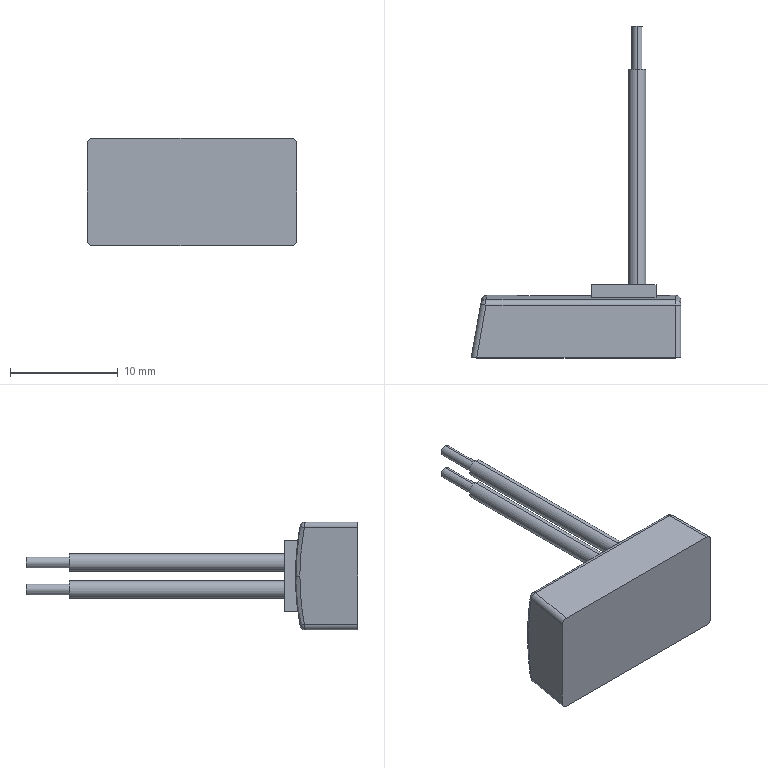Part | STEP file | 11-sy5120-5gz-01_v100 cover-V2.0-V2.011_G | 1 solid | 36 faces | box 19.45 x 30.8 x 10 mm | volume 1193 mm3 | cylinder 15 | plane 14 | sphere 4 | spline 2 | torus 1 | commonest cylinder face diameters 1 x10 1.6 x4 50 x1
STEP:
#1=CARTESIAN_POINT('',(-4.05,30.8,-0.75));
#2=VERTEX_POINT('',#1);
#3=CARTESIAN_POINT('',(-4.05,30.8,-1.75));
#4=VERTEX_POINT('',#3);
#5=CARTESIAN_POINT('',(-4.05,30.8,-1.25));
#6=DIRECTION('',(0.,1.,0.));
#7=DIRECTION('',(0.,0.,1.));
#8=AXIS2_PLACEMENT_3D('',#5,#6,#7);
#9=CIRCLE('',#8,0.5);
#10=EDGE_CURVE('',#2,#4,#9,.T.);
#11=ORIENTED_EDGE('',*,*,#10,.F.);
#12=CARTESIAN_POINT('',(-4.05,26.8,-0.75));
#13=VERTEX_POINT('',#12);
#14=CARTESIAN_POINT('',(-4.05,30.8,-0.75));
#15=DIRECTION('',(0.,-1.,0.));
#16=VECTOR('',#15,1000.);
#17=LINE('',#14,#16);
#18=EDGE_CURVE('',#2,#13,#17,.T.);
#19=ORIENTED_EDGE('',*,*,#18,.T.);
#20=CARTESIAN_POINT('',(-4.05,26.8,-1.75));
#21=VERTEX_POINT('',#20);
#22=CARTESIAN_POINT('',(-4.05,26.8,-1.25));
#23=DIRECTION('',(0.,1.,0.));
#24=DIRECTION('',(0.,0.,1.));
#25=AXIS2_PLACEMENT_3D('',#22,#23,#24);
#26=CIRCLE('',#25,0.5);
#27=EDGE_CURVE('',#13,#21,#26,.T.);
#28=ORIENTED_EDGE('',*,*,#27,.T.);
#29=CARTESIAN_POINT('',(-4.05,30.8,-1.75));
#30=DIRECTION('',(0.,-1.,0.));
#31=VECTOR('',#30,1000.);
#32=LINE('',#29,#31);
#33=EDGE_CURVE('',#4,#21,#32,.T.);
#34=ORIENTED_EDGE('',*,*,#33,.F.);
#35=EDGE_LOOP('',(#11,#19,#28,#34));
#36=FACE_OUTER_BOUND('',#35,.T.);
#37=CARTESIAN_POINT('',(-4.05,30.8,-1.25));
#38=DIRECTION('',(0.,-1.,0.));
#39=DIRECTION('',(0.,0.,-1.));
#40=AXIS2_PLACEMENT_3D('',#37,#38,#39);
#41=CYLINDRICAL_SURFACE('',#40,0.5);
#42=ADVANCED_FACE('',(#36),#41,.T.);
#43=CARTESIAN_POINT('',(-4.05,30.8,1.75));
#44=VERTEX_POINT('',#43);
#45=CARTESIAN_POINT('',(-4.05,30.8,0.75));
#46=VERTEX_POINT('',#45);
#47=CARTESIAN_POINT('',(-4.05,30.8,1.25));
#48=DIRECTION('',(0.,1.,0.));
#49=DIRECTION('',(0.,0.,1.));
#50=AXIS2_PLACEMENT_3D('',#47,#48,#49);
#51=CIRCLE('',#50,0.5);
#52=EDGE_CURVE('',#44,#46,#51,.T.);
#53=ORIENTED_EDGE('',*,*,#52,.F.);
#54=CARTESIAN_POINT('',(-4.05,26.8,1.75));
#55=VERTEX_POINT('',#54);
#56=CARTESIAN_POINT('',(-4.05,30.8,1.75));
#57=DIRECTION('',(0.,-1.,0.));
#58=VECTOR('',#57,1000.);
#59=LINE('',#56,#58);
#60=EDGE_CURVE('',#44,#55,#59,.T.);
#61=ORIENTED_EDGE('',*,*,#60,.T.);
#62=CARTESIAN_POINT('',(-4.05,26.8,0.75));
#63=VERTEX_POINT('',#62);
#64=CARTESIAN_POINT('',(-4.05,26.8,1.25));
#65=DIRECTION('',(0.,1.,0.));
#66=DIRECTION('',(0.,0.,1.));
#67=AXIS2_PLACEMENT_3D('',#64,#65,#66);
#68=CIRCLE('',#67,0.5);
#69=EDGE_CURVE('',#55,#63,#68,.T.);
#70=ORIENTED_EDGE('',*,*,#69,.T.);
#71=CARTESIAN_POINT('',(-4.05,30.8,0.75));
#72=DIRECTION('',(0.,-1.,0.));
#73=VECTOR('',#72,1000.);
#74=LINE('',#71,#73);
#75=EDGE_CURVE('',#46,#63,#74,.T.);
#76=ORIENTED_EDGE('',*,*,#75,.F.);
#77=EDGE_LOOP('',(#53,#61,#70,#76));
#78=FACE_OUTER_BOUND('',#77,.T.);
#79=CARTESIAN_POINT('',(-4.05,30.8,1.25));
#80=DIRECTION('',(0.,-1.,0.));
#81=DIRECTION('',(0.,0.,-1.));
#82=AXIS2_PLACEMENT_3D('',#79,#80,#81);
#83=CYLINDRICAL_SURFACE('',#82,0.5);
#84=ADVANCED_FACE('',(#78),#83,.T.);
#85=CARTESIAN_POINT('',(-4.05,26.8,-0.45));
#86=VERTEX_POINT('',#85);
#87=CARTESIAN_POINT('',(-4.05,26.8,-2.05));
#88=VERTEX_POINT('',#87);
#89=CARTESIAN_POINT('',(-4.05,26.8,-1.25));
#90=DIRECTION('',(0.,1.,0.));
#91=DIRECTION('',(0.,0.,1.));
#92=AXIS2_PLACEMENT_3D('',#89,#90,#91);
#93=CIRCLE('',#92,0.8);
#94=EDGE_CURVE('',#86,#88,#93,.T.);
#95=ORIENTED_EDGE('',*,*,#94,.F.);
#96=CARTESIAN_POINT('',(-4.05,6.8,-0.45));
#97=VERTEX_POINT('',#96);
#98=CARTESIAN_POINT('',(-4.05,26.8,-0.45));
#99=DIRECTION('',(0.,-1.,0.));
#100=VECTOR('',#99,1000.);
#101=LINE('',#98,#100);
#102=EDGE_CURVE('',#86,#97,#101,.T.);
#103=ORIENTED_EDGE('',*,*,#102,.T.);
#104=CARTESIAN_POINT('',(-4.05,6.8,-2.05));
#105=VERTEX_POINT('',#104);
#106=CARTESIAN_POINT('',(-4.05,6.8,-1.25));
#107=DIRECTION('',(0.,1.,0.));
#108=DIRECTION('',(0.,0.,-1.));
#109=AXIS2_PLACEMENT_3D('',#106,#107,#108);
#110=CIRCLE('',#109,0.8);
#111=EDGE_CURVE('',#97,#105,#110,.T.);
#112=ORIENTED_EDGE('',*,*,#111,.T.);
#113=CARTESIAN_POINT('',(-4.05,26.8,-2.05));
#114=DIRECTION('',(0.,-1.,0.));
#115=VECTOR('',#114,1000.);
#116=LINE('',#113,#115);
#117=EDGE_CURVE('',#88,#105,#116,.T.);
#118=ORIENTED_EDGE('',*,*,#117,.F.);
#119=EDGE_LOOP('',(#95,#103,#112,#118));
#120=FACE_OUTER_BOUND('',#119,.T.);
#121=CARTESIAN_POINT('',(-4.05,26.8,-1.25));
#122=DIRECTION('',(0.,-1.,0.));
#123=DIRECTION('',(0.,0.,-1.));
#124=AXIS2_PLACEMENT_3D('',#121,#122,#123);
#125=CYLINDRICAL_SURFACE('',#124,0.8);
#126=ADVANCED_FACE('',(#120),#125,.T.);
#127=CARTESIAN_POINT('',(-4.05,26.8,2.05));
#128=VERTEX_POINT('',#127);
#129=CARTESIAN_POINT('',(-4.05,26.8,0.45));
#130=VERTEX_POINT('',#129);
#131=CARTESIAN_POINT('',(-4.05,26.8,1.25));
#132=DIRECTION('',(0.,1.,0.));
#133=DIRECTION('',(0.,0.,1.));
#134=AXIS2_PLACEMENT_3D('',#131,#132,#133);
#135=CIRCLE('',#134,0.8);
#136=EDGE_CURVE('',#128,#130,#135,.T.);
#137=ORIENTED_EDGE('',*,*,#136,.F.);
#138=CARTESIAN_POINT('',(-4.05,6.8,2.05));
#139=VERTEX_POINT('',#138);
#140=CARTESIAN_POINT('',(-4.05,26.8,2.05));
#141=DIRECTION('',(0.,-1.,0.));
#142=VECTOR('',#141,1000.);
#143=LINE('',#140,#142);
#144=EDGE_CURVE('',#128,#139,#143,.T.);
#145=ORIENTED_EDGE('',*,*,#144,.T.);
#146=CARTESIAN_POINT('',(-4.05,6.8,0.45));
#147=VERTEX_POINT('',#146);
#148=CARTESIAN_POINT('',(-4.05,6.8,1.25));
#149=DIRECTION('',(0.,1.,0.));
#150=DIRECTION('',(0.,0.,-1.));
#151=AXIS2_PLACEMENT_3D('',#148,#149,#150);
#152=CIRCLE('',#151,0.8);
#153=EDGE_CURVE('',#139,#147,#152,.T.);
#154=ORIENTED_EDGE('',*,*,#153,.T.);
#155=CARTESIAN_POINT('',(-4.05,26.8,0.45));
#156=DIRECTION('',(0.,-1.,0.));
#157=VECTOR('',#156,1000.);
#158=LINE('',#155,#157);
#159=EDGE_CURVE('',#130,#147,#158,.T.);
#160=ORIENTED_EDGE('',*,*,#159,.F.);
#161=EDGE_LOOP('',(#137,#145,#154,#160));
#162=FACE_OUTER_BOUND('',#161,.T.);
#163=CARTESIAN_POINT('',(-4.05,26.8,1.25));
#164=DIRECTION('',(0.,-1.,0.));
#165=DIRECTION('',(0.,0.,-1.));
#166=AXIS2_PLACEMENT_3D('',#163,#164,#165);
#167=CYLINDRICAL_SURFACE('',#166,0.8);
#168=ADVANCED_FACE('',(#162),#167,.T.);
#169=CARTESIAN_POINT('',(-18.008,5.8,0.));
#170=VERTEX_POINT('',#169);
#171=CARTESIAN_POINT('',(-18.081,5.375,4.592));
#172=VERTEX_POINT('',#171);
#173=CARTESIAN_POINT('',(-18.008,5.8,0.));
#174=CARTESIAN_POINT('',(-18.008,5.8,1.542));
#175=CARTESIAN_POINT('',(-18.032,5.658,3.077));
#176=CARTESIAN_POINT('',(-18.081,5.375,4.592));
#177=(BOUNDED_CURVE()B_SPLINE_CURVE(3,(#173,#174,#175,#176),.UNSPECIFIED.,.F.,.F.)B_SPLINE_CURVE_WITH_KNOTS((4,4),(0.,0.1847),.UNSPECIFIED.)CURVE()GEOMETRIC_REPRESENTATION_ITEM()RATIONAL_B_SPLINE_CURVE((1.,0.9972,0.9972,1.))REPRESENTATION_ITEM(''));
#178=EDGE_CURVE('',#170,#172,#177,.T.);
#179=ORIENTED_EDGE('',*,*,#178,.F.);
#180=CARTESIAN_POINT('',(-18.5,5.387,0.));
#181=VERTEX_POINT('',#180);
#182=CARTESIAN_POINT('',(-18.008,5.3,0.));
#183=DIRECTION('',(0.,0.,1.));
#184=DIRECTION('',(1.,0.,0.));
#185=AXIS2_PLACEMENT_3D('',#182,#183,#184);
#186=CIRCLE('',#185,0.5);
#187=EDGE_CURVE('',#170,#181,#186,.T.);
#188=ORIENTED_EDGE('',*,*,#187,.T.);
#189=CARTESIAN_POINT('',(-18.574,4.97,4.5));
#190=VERTEX_POINT('',#189);
#191=CARTESIAN_POINT('',(-18.574,4.97,4.5));
#192=CARTESIAN_POINT('',(-18.525,5.247,3.015));
#193=CARTESIAN_POINT('',(-18.5,5.387,1.511));
#194=CARTESIAN_POINT('',(-18.5,5.387,0.));
#195=(BOUNDED_CURVE()B_SPLINE_CURVE(3,(#191,#192,#193,#194),.UNSPECIFIED.,.F.,.F.)B_SPLINE_CURVE_WITH_KNOTS((4,4),(6.098,6.283),.UNSPECIFIED.)CURVE()GEOMETRIC_REPRESENTATION_ITEM()RATIONAL_B_SPLINE_CURVE((1.,0.9972,0.9972,1.))REPRESENTATION_ITEM(''));
#196=EDGE_CURVE('',#190,#181,#195,.T.);
#197=ORIENTED_EDGE('',*,*,#196,.F.);
#198=CARTESIAN_POINT('',(-18.081,4.883,4.5));
#199=DIRECTION('',(0.03237,0.1836,-0.9825));
#200=DIRECTION('',(0.,-0.983,-0.1837));
#201=AXIS2_PLACEMENT_3D('',#198,#199,#200);
#202=CIRCLE('',#201,0.5);
#203=EDGE_CURVE('',#190,#172,#202,.T.);
#204=ORIENTED_EDGE('',*,*,#203,.T.);
#205=EDGE_LOOP('',(#179,#188,#197,#204));
#206=FACE_OUTER_BOUND('',#205,.T.);
#207=CARTESIAN_POINT('',(-18.081,5.375,4.592));
#208=CARTESIAN_POINT('',(-18.502,5.377,4.578));
#209=CARTESIAN_POINT('',(-18.574,4.97,4.5));
#210=CARTESIAN_POINT('',(-18.032,5.657,3.079));
#211=CARTESIAN_POINT('',(-18.452,5.658,3.071));
#212=CARTESIAN_POINT('',(-18.525,5.247,3.017));
#213=CARTESIAN_POINT('',(-18.008,5.8,1.539));
#214=CARTESIAN_POINT('',(-18.427,5.8,1.535));
#215=CARTESIAN_POINT('',(-18.5,5.387,1.509));
#216=CARTESIAN_POINT('',(-18.008,5.8,0.));
#217=CARTESIAN_POINT('',(-18.427,5.8,0.));
#218=CARTESIAN_POINT('',(-18.5,5.387,0.));
#219=(BOUNDED_SURFACE()B_SPLINE_SURFACE(3,2,((#207,#208,#209),(#210,#211,#212),(#213,#214,#215),(#216,#217,#218)),.UNSPECIFIED.,.F.,.F.,.F.)B_SPLINE_SURFACE_WITH_KNOTS((4,4),(3,3),(6.098,6.283),(0.,1.),.UNSPECIFIED.)GEOMETRIC_REPRESENTATION_ITEM()RATIONAL_B_SPLINE_SURFACE(((1.,0.7651,1.),(1.,0.7657,1.),(1.,0.766,1.),(1.,0.766,1.)))REPRESENTATION_ITEM('')SURFACE());
#220=ADVANCED_FACE('',(#206),#219,.T.);
#221=CARTESIAN_POINT('',(-4.05,26.8,-1.25));
#222=DIRECTION('',(0.,1.,0.));
#223=DIRECTION('',(0.,0.,1.));
#224=AXIS2_PLACEMENT_3D('',#221,#222,#223);
#225=CIRCLE('',#224,0.8);
#226=EDGE_CURVE('',#88,#86,#225,.T.);
#227=ORIENTED_EDGE('',*,*,#226,.T.);
#228=ORIENTED_EDGE('',*,*,#94,.T.);
#229=EDGE_LOOP('',(#227,#228));
#230=FACE_OUTER_BOUND('',#229,.T.);
#231=CARTESIAN_POINT('',(-4.05,26.8,-1.25));
#232=DIRECTION('',(0.,1.,0.));
#233=DIRECTION('',(0.,0.,1.));
#234=AXIS2_PLACEMENT_3D('',#231,#232,#233);
#235=CIRCLE('',#234,0.5);
#236=EDGE_CURVE('',#21,#13,#235,.T.);
#237=ORIENTED_EDGE('',*,*,#236,.F.);
#238=ORIENTED_EDGE('',*,*,#27,.F.);
#239=EDGE_LOOP('',(#237,#238));
#240=FACE_BOUND('',#239,.T.);
#241=CARTESIAN_POINT('',(-4.05,26.8,-1.25));
#242=DIRECTION('',(0.,1.,0.));
#243=DIRECTION('',(0.,0.,1.));
#244=AXIS2_PLACEMENT_3D('',#241,#242,#243);
#245=PLANE('',#244);
#246=ADVANCED_FACE('',(#230,#240),#245,.T.);
#247=CARTESIAN_POINT('',(-4.05,26.8,1.25));
#248=DIRECTION('',(0.,1.,0.));
#249=DIRECTION('',(0.,0.,1.));
#250=AXIS2_PLACEMENT_3D('',#247,#248,#249);
#251=CIRCLE('',#250,0.8);
#252=EDGE_CURVE('',#130,#128,#251,.T.);
#253=ORIENTED_EDGE('',*,*,#252,.T.);
#254=ORIENTED_EDGE('',*,*,#136,.T.);
#255=EDGE_LOOP('',(#253,#254));
#256=FACE_OUTER_BOUND('',#255,.T.);
#257=CARTESIAN_POINT('',(-4.05,26.8,1.25));
#258=DIRECTION('',(0.,1.,0.));
#259=DIRECTION('',(0.,0.,1.));
#260=AXIS2_PLACEMENT_3D('',#257,#258,#259);
#261=CIRCLE('',#260,0.5);
#262=EDGE_CURVE('',#63,#55,#261,.T.);
#263=ORIENTED_EDGE('',*,*,#262,.F.);
#264=ORIENTED_EDGE('',*,*,#69,.F.);
#265=EDGE_LOOP('',(#263,#264));
#266=FACE_BOUND('',#265,.T.);
#267=CARTESIAN_POINT('',(-4.05,26.8,1.25));
#268=DIRECTION('',(0.,1.,0.));
#269=DIRECTION('',(0.,0.,1.));
#270=AXIS2_PLACEMENT_3D('',#267,#268,#269);
#271=PLANE('',#270);
#272=ADVANCED_FACE('',(#256,#266),#271,.T.);
#273=CARTESIAN_POINT('',(-4.05,6.8,1.25));
#274=DIRECTION('',(0.,1.,0.));
#275=DIRECTION('',(0.,0.,-1.));
#276=AXIS2_PLACEMENT_3D('',#273,#274,#275);
#277=CIRCLE('',#276,0.8);
#278=EDGE_CURVE('',#147,#139,#277,.T.);
#279=ORIENTED_EDGE('',*,*,#278,.F.);
#280=ORIENTED_EDGE('',*,*,#153,.F.);
#281=EDGE_LOOP('',(#279,#280));
#282=FACE_BOUND('',#281,.T.);
#283=CARTESIAN_POINT('',(-8.3,6.8,3.3));
#284=VERTEX_POINT('',#283);
#285=CARTESIAN_POINT('',(-8.3,6.8,-3.3));
#286=VERTEX_POINT('',#285);
#287=CARTESIAN_POINT('',(-8.3,6.8,3.3));
#288=DIRECTION('',(0.,0.,-1.));
#289=VECTOR('',#288,1000.);
#290=LINE('',#287,#289);
#291=EDGE_CURVE('',#284,#286,#290,.T.);
#292=ORIENTED_EDGE('',*,*,#291,.F.);
#293=CARTESIAN_POINT('',(-2.3,6.8,3.3));
#294=VERTEX_POINT('',#293);
#295=CARTESIAN_POINT('',(-8.3,6.8,3.3));
#296=DIRECTION('',(-1.,0.,0.));
#297=VECTOR('',#296,1000.);
#298=LINE('',#295,#297);
#299=EDGE_CURVE('',#294,#284,#298,.T.);
#300=ORIENTED_EDGE('',*,*,#299,.F.);
#301=CARTESIAN_POINT('',(-2.3,6.8,-3.3));
#302=VERTEX_POINT('',#301);
#303=CARTESIAN_POINT('',(-2.3,6.8,3.3));
#304=DIRECTION('',(0.,0.,1.));
#305=VECTOR('',#304,1000.);
#306=LINE('',#303,#305);
#307=EDGE_CURVE('',#302,#294,#306,.T.);
#308=ORIENTED_EDGE('',*,*,#307,.F.);
#309=CARTESIAN_POINT('',(-8.3,6.8,-3.3));
#310=DIRECTION('',(1.,0.,0.));
#311=VECTOR('',#310,1000.);
#312=LINE('',#309,#311);
#313=EDGE_CURVE('',#286,#302,#312,.T.);
#314=ORIENTED_EDGE('',*,*,#313,.F.);
#315=EDGE_LOOP('',(#292,#300,#308,#314));
#316=FACE_OUTER_BOUND('',#315,.T.);
#317=CARTESIAN_POINT('',(-4.05,6.8,-1.25));
#318=DIRECTION('',(0.,1.,0.));
#319=DIRECTION('',(0.,0.,-1.));
#320=AXIS2_PLACEMENT_3D('',#317,#318,#319);
#321=CIRCLE('',#320,0.8);
#322=EDGE_CURVE('',#105,#97,#321,.T.);
#323=ORIENTED_EDGE('',*,*,#322,.F.);
#324=ORIENTED_EDGE('',*,*,#111,.F.);
#325=EDGE_LOOP('',(#323,#324));
#326=FACE_BOUND('',#325,.T.);
#327=CARTESIAN_POINT('',(-8.3,6.8,-3.3));
#328=DIRECTION('',(0.,-1.,0.));
#329=DIRECTION('',(0.,0.,-1.));
#330=AXIS2_PLACEMENT_3D('',#327,#328,#329);
#331=PLANE('',#330);
#332=ADVANCED_FACE('',(#282,#316,#326),#331,.F.);
#333=CARTESIAN_POINT('',(-18.942,0.,5.));
#334=VERTEX_POINT('',#333);
#335=CARTESIAN_POINT('',(-0.5,0.,5.));
#336=VERTEX_POINT('',#335);
#337=CARTESIAN_POINT('',(-19.45,0.,5.));
#338=DIRECTION('',(1.,0.,0.));
#339=VECTOR('',#338,1000.);
#340=LINE('',#337,#339);
#341=EDGE_CURVE('',#334,#336,#340,.T.);
#342=ORIENTED_EDGE('',*,*,#341,.T.);
#343=CARTESIAN_POINT('',(-0.5,4.883,5.));
#344=VERTEX_POINT('',#343);
#345=CARTESIAN_POINT('',(-0.5,0.,5.));
#346=DIRECTION('',(0.,1.,0.));
#347=VECTOR('',#346,1000.);
#348=LINE('',#345,#347);
#349=EDGE_CURVE('',#336,#344,#348,.T.);
#350=ORIENTED_EDGE('',*,*,#349,.T.);
#351=CARTESIAN_POINT('',(-18.081,4.883,5.));
#352=VERTEX_POINT('',#351);
#353=CARTESIAN_POINT('',(-19.45,4.883,5.));
#354=DIRECTION('',(-1.,0.,0.));
#355=VECTOR('',#354,1000.);
#356=LINE('',#353,#355);
#357=EDGE_CURVE('',#344,#352,#356,.T.);
#358=ORIENTED_EDGE('',*,*,#357,.T.);
#359=CARTESIAN_POINT('',(-18.958,-0.08682,5.));
#360=DIRECTION('',(-0.1736,-0.9848,0.));
#361=VECTOR('',#360,1000.);
#362=LINE('',#359,#361);
#363=EDGE_CURVE('',#352,#334,#362,.T.);
#364=ORIENTED_EDGE('',*,*,#363,.T.);
#365=EDGE_LOOP('',(#342,#350,#358,#364));
#366=FACE_OUTER_BOUND('',#365,.T.);
#367=CARTESIAN_POINT('',(-19.45,0.,5.));
#368=DIRECTION('',(0.,0.,1.));
#369=DIRECTION('',(1.,0.,0.));
#370=AXIS2_PLACEMENT_3D('',#367,#368,#369);
#371=PLANE('',#370);
#372=ADVANCED_FACE('',(#366),#371,.T.);
#373=CARTESIAN_POINT('',(-8.3,5.581,-3.3));
#374=VERTEX_POINT('',#373);
#375=CARTESIAN_POINT('',(-8.3,5.581,3.3));
#376=VERTEX_POINT('',#375);
#377=CARTESIAN_POINT('',(-8.3,-19.2,0.));
#378=DIRECTION('',(1.,0.,0.));
#379=DIRECTION('',(0.,0.,1.));
#380=AXIS2_PLACEMENT_3D('',#377,#378,#379);
#381=CIRCLE('',#380,25.);
#382=EDGE_CURVE('',#374,#376,#381,.T.);
#383=ORIENTED_EDGE('',*,*,#382,.F.);
#384=CARTESIAN_POINT('',(-2.3,5.581,-3.3));
#385=VERTEX_POINT('',#384);
#386=CARTESIAN_POINT('',(-19.45,5.581,-3.3));
#387=DIRECTION('',(-1.,0.,0.));
#388=VECTOR('',#387,1000.);
#389=LINE('',#386,#388);
#390=EDGE_CURVE('',#385,#374,#389,.T.);
#391=ORIENTED_EDGE('',*,*,#390,.F.);
#392=CARTESIAN_POINT('',(-2.3,5.581,3.3));
#393=VERTEX_POINT('',#392);
#394=CARTESIAN_POINT('',(-2.3,-19.2,0.));
#395=DIRECTION('',(-1.,0.,0.));
#396=DIRECTION('',(0.,0.,-1.));
#397=AXIS2_PLACEMENT_3D('',#394,#395,#396);
#398=CIRCLE('',#397,25.);
#399=EDGE_CURVE('',#393,#385,#398,.T.);
#400=ORIENTED_EDGE('',*,*,#399,.F.);
#401=CARTESIAN_POINT('',(-19.45,5.581,3.3));
#402=DIRECTION('',(1.,0.,0.));
#403=VECTOR('',#402,1000.);
#404=LINE('',#401,#403);
#405=EDGE_CURVE('',#376,#393,#404,.T.);
#406=ORIENTED_EDGE('',*,*,#405,.F.);
#407=EDGE_LOOP('',(#383,#391,#400,#406));
#408=FACE_BOUND('',#407,.T.);
#409=CARTESIAN_POINT('',(-0.5,5.375,-4.592));
#410=VERTEX_POINT('',#409);
#411=CARTESIAN_POINT('',(-18.081,5.375,-4.592));
#412=VERTEX_POINT('',#411);
#413=CARTESIAN_POINT('',(-19.45,5.375,-4.592));
#414=DIRECTION('',(-1.,0.,0.));
#415=VECTOR('',#414,1000.);
#416=LINE('',#413,#415);
#417=EDGE_CURVE('',#410,#412,#416,.T.);
#418=ORIENTED_EDGE('',*,*,#417,.T.);
#419=CARTESIAN_POINT('',(-18.081,5.375,-4.592));
#420=CARTESIAN_POINT('',(-18.032,5.658,-3.077));
#421=CARTESIAN_POINT('',(-18.008,5.8,-1.542));
#422=CARTESIAN_POINT('',(-18.008,5.8,0.));
#423=(BOUNDED_CURVE()B_SPLINE_CURVE(3,(#419,#420,#421,#422),.UNSPECIFIED.,.F.,.F.)B_SPLINE_CURVE_WITH_KNOTS((4,4),(6.098,6.283),.UNSPECIFIED.)CURVE()GEOMETRIC_REPRESENTATION_ITEM()RATIONAL_B_SPLINE_CURVE((1.,0.9972,0.9972,1.))REPRESENTATION_ITEM(''));
#424=EDGE_CURVE('',#412,#170,#423,.T.);
#425=ORIENTED_EDGE('',*,*,#424,.T.);
#426=ORIENTED_EDGE('',*,*,#178,.T.);
#427=CARTESIAN_POINT('',(-0.5,5.375,4.592));
#428=VERTEX_POINT('',#427);
#429=CARTESIAN_POINT('',(-19.45,5.375,4.592));
#430=DIRECTION('',(1.,0.,0.));
#431=VECTOR('',#430,1000.);
#432=LINE('',#429,#431);
#433=EDGE_CURVE('',#172,#428,#432,.T.);
#434=ORIENTED_EDGE('',*,*,#433,.T.);
#435=CARTESIAN_POINT('',(-0.5,-19.2,0.));
#436=DIRECTION('',(-1.,0.,0.));
#437=DIRECTION('',(0.,0.,-1.));
#438=AXIS2_PLACEMENT_3D('',#435,#436,#437);
#439=CIRCLE('',#438,25.);
#440=EDGE_CURVE('',#428,#410,#439,.T.);
#441=ORIENTED_EDGE('',*,*,#440,.T.);
#442=EDGE_LOOP('',(#418,#425,#426,#434,#441));
#443=FACE_OUTER_BOUND('',#442,.T.);
#444=CARTESIAN_POINT('',(-19.45,-19.2,0.));
#445=DIRECTION('',(1.,0.,0.));
#446=DIRECTION('',(0.,0.,-1.));
#447=AXIS2_PLACEMENT_3D('',#444,#445,#446);
#448=CYLINDRICAL_SURFACE('',#447,25.);
#449=ADVANCED_FACE('',(#408,#443),#448,.T.);
#450=CARTESIAN_POINT('',(-18.942,0.,-5.));
#451=VERTEX_POINT('',#450);
#452=CARTESIAN_POINT('',(-0.5,0.,-5.));
#453=VERTEX_POINT('',#452);
#454=CARTESIAN_POINT('',(-19.45,0.,-5.));
#455=DIRECTION('',(1.,0.,0.));
#456=VECTOR('',#455,1000.);
#457=LINE('',#454,#456);
#458=EDGE_CURVE('',#451,#453,#457,.T.);
#459=ORIENTED_EDGE('',*,*,#458,.F.);
#460=CARTESIAN_POINT('',(-18.081,4.883,-5.));
#461=VERTEX_POINT('',#460);
#462=CARTESIAN_POINT('',(-18.024,5.208,-5.));
#463=DIRECTION('',(0.1736,0.9848,0.));
#464=VECTOR('',#463,1000.);
#465=LINE('',#462,#464);
#466=EDGE_CURVE('',#451,#461,#465,.T.);
#467=ORIENTED_EDGE('',*,*,#466,.T.);
#468=CARTESIAN_POINT('',(-0.5,4.883,-5.));
#469=VERTEX_POINT('',#468);
#470=CARTESIAN_POINT('',(-19.45,4.883,-5.));
#471=DIRECTION('',(1.,0.,0.));
#472=VECTOR('',#471,1000.);
#473=LINE('',#470,#472);
#474=EDGE_CURVE('',#461,#469,#473,.T.);
#475=ORIENTED_EDGE('',*,*,#474,.T.);
#476=CARTESIAN_POINT('',(-0.5,0.,-5.));
#477=DIRECTION('',(0.,-1.,0.));
#478=VECTOR('',#477,1000.);
#479=LINE('',#476,#478);
#480=EDGE_CURVE('',#469,#453,#479,.T.);
#481=ORIENTED_EDGE('',*,*,#480,.T.);
#482=EDGE_LOOP('',(#459,#467,#475,#481));
#483=FACE_OUTER_BOUND('',#482,.T.);
#484=CARTESIAN_POINT('',(-19.45,0.,-5.));
#485=DIRECTION('',(0.,0.,-1.));
#486=DIRECTION('',(-1.,0.,0.));
#487=AXIS2_PLACEMENT_3D('',#484,#485,#486);
#488=PLANE('',#487);
#489=ADVANCED_FACE('',(#483),#488,.T.);
#490=CARTESIAN_POINT('',(-19.45,0.,4.5));
#491=VERTEX_POINT('',#490);
#492=CARTESIAN_POINT('',(-19.45,0.,-4.5));
#493=VERTEX_POINT('',#492);
#494=CARTESIAN_POINT('',(-19.45,0.,5.));
#495=DIRECTION('',(0.,0.,-1.));
#496=VECTOR('',#495,1000.);
#497=LINE('',#494,#496);
#498=EDGE_CURVE('',#491,#493,#497,.T.);
#499=ORIENTED_EDGE('',*,*,#498,.T.);
#500=CARTESIAN_POINT('',(-19.45,0.,-4.5));
#501=CARTESIAN_POINT('',(-19.45,0.,-4.793));
#502=CARTESIAN_POINT('',(-19.24,0.,-5.));
#503=CARTESIAN_POINT('',(-18.942,0.,-5.));
#504=(BOUNDED_CURVE()B_SPLINE_CURVE(3,(#500,#501,#502,#503),.UNSPECIFIED.,.F.,.F.)B_SPLINE_CURVE_WITH_KNOTS((4,4),(3.142,4.712),.UNSPECIFIED.)CURVE()GEOMETRIC_REPRESENTATION_ITEM()RATIONAL_B_SPLINE_CURVE((1.,0.8047,0.8047,1.))REPRESENTATION_ITEM(''));
#505=EDGE_CURVE('',#493,#451,#504,.T.);
#506=ORIENTED_EDGE('',*,*,#505,.T.);
#507=ORIENTED_EDGE('',*,*,#458,.T.);
#508=CARTESIAN_POINT('',(0.,0.,-4.5));
#509=VERTEX_POINT('',#508);
#510=CARTESIAN_POINT('',(-0.5,0.,-4.5));
#511=DIRECTION('',(0.,-1.,0.));
#512=DIRECTION('',(0.,0.,-1.));
#513=AXIS2_PLACEMENT_3D('',#510,#511,#512);
#514=CIRCLE('',#513,0.5);
#515=EDGE_CURVE('',#453,#509,#514,.T.);
#516=ORIENTED_EDGE('',*,*,#515,.T.);
#517=CARTESIAN_POINT('',(0.,0.,4.5));
#518=VERTEX_POINT('',#517);
#519=CARTESIAN_POINT('',(0.,0.,5.));
#520=DIRECTION('',(0.,0.,-1.));
#521=VECTOR('',#520,1000.);
#522=LINE('',#519,#521);
#523=EDGE_CURVE('',#518,#509,#522,.T.);
#524=ORIENTED_EDGE('',*,*,#523,.F.);
#525=CARTESIAN_POINT('',(-0.5,0.,4.5));
#526=DIRECTION('',(0.,-1.,0.));
#527=DIRECTION('',(0.,0.,-1.));
#528=AXIS2_PLACEMENT_3D('',#525,#526,#527);
#529=CIRCLE('',#528,0.5);
#530=EDGE_CURVE('',#518,#336,#529,.T.);
#531=ORIENTED_EDGE('',*,*,#530,.T.);
#532=ORIENTED_EDGE('',*,*,#341,.F.);
#533=CARTESIAN_POINT('',(-18.942,0.,5.));
#534=CARTESIAN_POINT('',(-19.24,0.,5.));
#535=CARTESIAN_POINT('',(-19.45,0.,4.793));
#536=CARTESIAN_POINT('',(-19.45,0.,4.5));
#537=(BOUNDED_CURVE()B_SPLINE_CURVE(3,(#533,#534,#535,#536),.UNSPECIFIED.,.F.,.F.)B_SPLINE_CURVE_WITH_KNOTS((4,4),(4.712,6.283),.UNSPECIFIED.)CURVE()GEOMETRIC_REPRESENTATION_ITEM()RATIONAL_B_SPLINE_CURVE((1.,0.8047,0.8047,1.))REPRESENTATION_ITEM(''));
#538=EDGE_CURVE('',#334,#491,#537,.T.);
#539=ORIENTED_EDGE('',*,*,#538,.T.);
#540=EDGE_LOOP('',(#499,#506,#507,#516,#524,#531,#532,#539));
#541=FACE_OUTER_BOUND('',#540,.T.);
#542=CARTESIAN_POINT('',(-19.45,0.,5.));
#543=DIRECTION('',(0.,-1.,0.));
#544=DIRECTION('',(0.,0.,-1.));
#545=AXIS2_PLACEMENT_3D('',#542,#543,#544);
#546=PLANE('',#545);
#547=ADVANCED_FACE('',(#541),#546,.T.);
#548=ORIENTED_EDGE('',*,*,#196,.T.);
#549=CARTESIAN_POINT('',(-18.574,4.97,-4.5));
#550=VERTEX_POINT('',#549);
#551=CARTESIAN_POINT('',(-18.5,5.387,0.));
#552=CARTESIAN_POINT('',(-18.5,5.387,-1.511));
#553=CARTESIAN_POINT('',(-18.525,5.247,-3.015));
#554=CARTESIAN_POINT('',(-18.574,4.97,-4.5));
#555=(BOUNDED_CURVE()B_SPLINE_CURVE(3,(#551,#552,#553,#554),.UNSPECIFIED.,.F.,.F.)B_SPLINE_CURVE_WITH_KNOTS((4,4),(0.,0.1847),.UNSPECIFIED.)CURVE()GEOMETRIC_REPRESENTATION_ITEM()RATIONAL_B_SPLINE_CURVE((1.,0.9972,0.9972,1.))REPRESENTATION_ITEM(''));
#556=EDGE_CURVE('',#181,#550,#555,.T.);
#557=ORIENTED_EDGE('',*,*,#556,.T.);
#558=CARTESIAN_POINT('',(-19.45,0.,-4.5));
#559=DIRECTION('',(-0.1736,-0.9848,0.));
#560=VECTOR('',#559,1000.);
#561=LINE('',#558,#560);
#562=EDGE_CURVE('',#550,#493,#561,.T.);
#563=ORIENTED_EDGE('',*,*,#562,.T.);
#564=ORIENTED_EDGE('',*,*,#498,.F.);
#565=CARTESIAN_POINT('',(-18.516,5.295,4.5));
#566=DIRECTION('',(0.1736,0.9848,0.));
#567=VECTOR('',#566,1000.);
#568=LINE('',#565,#567);
#569=EDGE_CURVE('',#491,#190,#568,.T.);
#570=ORIENTED_EDGE('',*,*,#569,.T.);
#571=EDGE_LOOP('',(#548,#557,#563,#564,#570));
#572=FACE_OUTER_BOUND('',#571,.T.);
#573=CARTESIAN_POINT('',(-19.45,0.,5.));
#574=DIRECTION('',(-0.9848,0.1736,0.));
#575=DIRECTION('',(-0.1736,-0.9848,0.));
#576=AXIS2_PLACEMENT_3D('',#573,#574,#575);
#577=PLANE('',#576);
#578=ADVANCED_FACE('',(#572),#577,.T.);
#579=ORIENTED_EDGE('',*,*,#523,.T.);
#580=CARTESIAN_POINT('',(0.,4.883,-4.5));
#581=VERTEX_POINT('',#580);
#582=CARTESIAN_POINT('',(0.,-19.2,-4.5));
#583=DIRECTION('',(0.,1.,0.));
#584=VECTOR('',#583,1000.);
#585=LINE('',#582,#584);
#586=EDGE_CURVE('',#509,#581,#585,.T.);
#587=ORIENTED_EDGE('',*,*,#586,.T.);
#588=CARTESIAN_POINT('',(0.,4.883,4.5));
#589=VERTEX_POINT('',#588);
#590=CARTESIAN_POINT('',(0.,-19.2,0.));
#591=DIRECTION('',(1.,0.,0.));
#592=DIRECTION('',(0.,0.,-1.));
#593=AXIS2_PLACEMENT_3D('',#590,#591,#592);
#594=CIRCLE('',#593,24.5);
#595=EDGE_CURVE('',#581,#589,#594,.T.);
#596=ORIENTED_EDGE('',*,*,#595,.T.);
#597=CARTESIAN_POINT('',(0.,-19.2,4.5));
#598=DIRECTION('',(0.,-1.,0.));
#599=VECTOR('',#598,1000.);
#600=LINE('',#597,#599);
#601=EDGE_CURVE('',#589,#518,#600,.T.);
#602=ORIENTED_EDGE('',*,*,#601,.T.);
#603=EDGE_LOOP('',(#579,#587,#596,#602));
#604=FACE_OUTER_BOUND('',#603,.T.);
#605=CARTESIAN_POINT('',(0.,-19.2,0.));
#606=DIRECTION('',(1.,0.,0.));
#607=DIRECTION('',(0.,0.,-1.));
#608=AXIS2_PLACEMENT_3D('',#605,#606,#607);
#609=PLANE('',#608);
#610=ADVANCED_FACE('',(#604),#609,.T.);
#611=CARTESIAN_POINT('',(-0.5,4.883,4.5));
#612=DIRECTION('',(0.,1.,0.));
#613=DIRECTION('',(-1.,0.,0.));
#614=AXIS2_PLACEMENT_3D('',#611,#612,#613);
#615=CIRCLE('',#614,0.5);
#616=EDGE_CURVE('',#344,#589,#615,.T.);
#617=ORIENTED_EDGE('',*,*,#616,.F.);
#618=ORIENTED_EDGE('',*,*,#349,.F.);
#619=ORIENTED_EDGE('',*,*,#530,.F.);
#620=ORIENTED_EDGE('',*,*,#601,.F.);
#621=EDGE_LOOP('',(#617,#618,#619,#620));
#622=FACE_OUTER_BOUND('',#621,.T.);
#623=CARTESIAN_POINT('',(-0.5,-19.2,4.5));
#624=DIRECTION('',(0.,-1.,0.));
#625=DIRECTION('',(0.,0.,-1.));
#626=AXIS2_PLACEMENT_3D('',#623,#624,#625);
#627=CYLINDRICAL_SURFACE('',#626,0.5);
#628=ADVANCED_FACE('',(#622),#627,.T.);
#629=CARTESIAN_POINT('',(-0.5,4.883,4.5));
#630=DIRECTION('',(-1.,0.,0.));
#631=DIRECTION('',(0.,0.,-1.));
#632=AXIS2_PLACEMENT_3D('',#629,#630,#631);
#633=CIRCLE('',#632,0.5);
#634=EDGE_CURVE('',#344,#428,#633,.T.);
#635=ORIENTED_EDGE('',*,*,#634,.F.);
#636=ORIENTED_EDGE('',*,*,#616,.T.);
#637=CARTESIAN_POINT('',(-0.5,4.883,4.5));
#638=DIRECTION('',(0.,0.1837,-0.983));
#639=DIRECTION('',(0.,-0.983,-0.1837));
#640=AXIS2_PLACEMENT_3D('',#637,#638,#639);
#641=CIRCLE('',#640,0.5);
#642=EDGE_CURVE('',#428,#589,#641,.T.);
#643=ORIENTED_EDGE('',*,*,#642,.F.);
#644=EDGE_LOOP('',(#635,#636,#643));
#645=FACE_OUTER_BOUND('',#644,.T.);
#646=CARTESIAN_POINT('',(-0.5,4.883,4.5));
#647=DIRECTION('',(0.,1.,0.));
#648=DIRECTION('',(1.,0.,0.));
#649=AXIS2_PLACEMENT_3D('',#646,#647,#648);
#650=SPHERICAL_SURFACE('',#649,0.5);
#651=ADVANCED_FACE('',(#645),#650,.T.);
#652=ORIENTED_EDGE('',*,*,#515,.F.);
#653=ORIENTED_EDGE('',*,*,#480,.F.);
#654=CARTESIAN_POINT('',(-0.5,4.883,-4.5));
#655=DIRECTION('',(0.,1.,0.));
#656=DIRECTION('',(0.,0.,1.));
#657=AXIS2_PLACEMENT_3D('',#654,#655,#656);
#658=CIRCLE('',#657,0.5);
#659=EDGE_CURVE('',#581,#469,#658,.T.);
#660=ORIENTED_EDGE('',*,*,#659,.F.);
#661=ORIENTED_EDGE('',*,*,#586,.F.);
#662=EDGE_LOOP('',(#652,#653,#660,#661));
#663=FACE_OUTER_BOUND('',#662,.T.);
#664=CARTESIAN_POINT('',(-0.5,-19.2,-4.5));
#665=DIRECTION('',(0.,1.,0.));
#666=DIRECTION('',(0.,0.,1.));
#667=AXIS2_PLACEMENT_3D('',#664,#665,#666);
#668=CYLINDRICAL_SURFACE('',#667,0.5);
#669=ADVANCED_FACE('',(#663),#668,.T.);
#670=ORIENTED_EDGE('',*,*,#642,.T.);
#671=ORIENTED_EDGE('',*,*,#595,.F.);
#672=CARTESIAN_POINT('',(-0.5,4.883,-4.5));
#673=DIRECTION('',(0.,-0.1837,-0.983));
#674=DIRECTION('',(0.,0.983,-0.1837));
#675=AXIS2_PLACEMENT_3D('',#672,#673,#674);
#676=CIRCLE('',#675,0.5);
#677=EDGE_CURVE('',#410,#581,#676,.T.);
#678=ORIENTED_EDGE('',*,*,#677,.F.);
#679=ORIENTED_EDGE('',*,*,#440,.F.);
#680=EDGE_LOOP('',(#670,#671,#678,#679));
#681=FACE_OUTER_BOUND('',#680,.T.);
#682=CARTESIAN_POINT('',(-0.5,-19.2,0.));
#683=DIRECTION('',(1.,0.,0.));
#684=DIRECTION('',(0.,0.,-1.));
#685=AXIS2_PLACEMENT_3D('',#682,#683,#684);
#686=TOROIDAL_SURFACE('',#685,24.5,0.5);
#687=ADVANCED_FACE('',(#681),#686,.T.);
#688=ORIENTED_EDGE('',*,*,#634,.T.);
#689=ORIENTED_EDGE('',*,*,#433,.F.);
#690=CARTESIAN_POINT('',(-18.081,4.883,4.5));
#691=DIRECTION('',(-1.,0.,0.));
#692=DIRECTION('',(0.,-1.,0.));
#693=AXIS2_PLACEMENT_3D('',#690,#691,#692);
#694=CIRCLE('',#693,0.5);
#695=EDGE_CURVE('',#352,#172,#694,.T.);
#696=ORIENTED_EDGE('',*,*,#695,.F.);
#697=ORIENTED_EDGE('',*,*,#357,.F.);
#698=EDGE_LOOP('',(#688,#689,#696,#697));
#699=FACE_OUTER_BOUND('',#698,.T.);
#700=CARTESIAN_POINT('',(-19.45,4.883,4.5));
#701=DIRECTION('',(1.,0.,0.));
#702=DIRECTION('',(0.,0.,-1.));
#703=AXIS2_PLACEMENT_3D('',#700,#701,#702);
#704=CYLINDRICAL_SURFACE('',#703,0.5);
#705=ADVANCED_FACE('',(#699),#704,.T.);
#706=ORIENTED_EDGE('',*,*,#538,.F.);
#707=ORIENTED_EDGE('',*,*,#363,.F.);
#708=CARTESIAN_POINT('',(-18.081,4.883,4.5));
#709=DIRECTION('',(0.1736,0.9848,0.));
#710=DIRECTION('',(-0.9848,0.1736,0.));
#711=AXIS2_PLACEMENT_3D('',#708,#709,#710);
#712=CIRCLE('',#711,0.5);
#713=EDGE_CURVE('',#190,#352,#712,.T.);
#714=ORIENTED_EDGE('',*,*,#713,.F.);
#715=ORIENTED_EDGE('',*,*,#569,.F.);
#716=EDGE_LOOP('',(#706,#707,#714,#715));
#717=FACE_OUTER_BOUND('',#716,.T.);
#718=CARTESIAN_POINT('',(-18.958,-0.08682,4.5));
#719=DIRECTION('',(-0.1736,-0.9848,0.));
#720=DIRECTION('',(0.9848,-0.1736,0.));
#721=AXIS2_PLACEMENT_3D('',#718,#719,#720);
#722=CYLINDRICAL_SURFACE('',#721,0.5);
#723=ADVANCED_FACE('',(#717),#722,.T.);
#724=ORIENTED_EDGE('',*,*,#677,.T.);
#725=ORIENTED_EDGE('',*,*,#659,.T.);
#726=CARTESIAN_POINT('',(-0.5,4.883,-4.5));
#727=DIRECTION('',(-1.,0.,0.));
#728=DIRECTION('',(0.,1.,0.));
#729=AXIS2_PLACEMENT_3D('',#726,#727,#728);
#730=CIRCLE('',#729,0.5);
#731=EDGE_CURVE('',#410,#469,#730,.T.);
#732=ORIENTED_EDGE('',*,*,#731,.F.);
#733=EDGE_LOOP('',(#724,#725,#732));
#734=FACE_OUTER_BOUND('',#733,.T.);
#735=CARTESIAN_POINT('',(-0.5,4.883,-4.5));
#736=DIRECTION('',(0.,1.,0.));
#737=DIRECTION('',(1.,0.,0.));
#738=AXIS2_PLACEMENT_3D('',#735,#736,#737);
#739=SPHERICAL_SURFACE('',#738,0.5);
#740=ADVANCED_FACE('',(#734),#739,.T.);
#741=ORIENTED_EDGE('',*,*,#713,.T.);
#742=ORIENTED_EDGE('',*,*,#695,.T.);
#743=ORIENTED_EDGE('',*,*,#203,.F.);
#744=EDGE_LOOP('',(#741,#742,#743));
#745=FACE_OUTER_BOUND('',#744,.T.);
#746=CARTESIAN_POINT('',(-18.081,4.883,4.5));
#747=DIRECTION('',(0.,1.,0.));
#748=DIRECTION('',(1.,0.,0.));
#749=AXIS2_PLACEMENT_3D('',#746,#747,#748);
#750=SPHERICAL_SURFACE('',#749,0.5);
#751=ADVANCED_FACE('',(#745),#750,.T.);
#752=ORIENTED_EDGE('',*,*,#731,.T.);
#753=ORIENTED_EDGE('',*,*,#474,.F.);
#754=CARTESIAN_POINT('',(-18.081,4.883,-4.5));
#755=DIRECTION('',(-1.,0.,0.));
#756=DIRECTION('',(0.,0.,1.));
#757=AXIS2_PLACEMENT_3D('',#754,#755,#756);
#758=CIRCLE('',#757,0.5);
#759=EDGE_CURVE('',#412,#461,#758,.T.);
#760=ORIENTED_EDGE('',*,*,#759,.F.);
#761=ORIENTED_EDGE('',*,*,#417,.F.);
#762=EDGE_LOOP('',(#752,#753,#760,#761));
#763=FACE_OUTER_BOUND('',#762,.T.);
#764=CARTESIAN_POINT('',(-19.45,4.883,-4.5));
#765=DIRECTION('',(1.,0.,0.));
#766=DIRECTION('',(0.,0.,-1.));
#767=AXIS2_PLACEMENT_3D('',#764,#765,#766);
#768=CYLINDRICAL_SURFACE('',#767,0.5);
#769=ADVANCED_FACE('',(#763),#768,.T.);
#770=ORIENTED_EDGE('',*,*,#187,.F.);
#771=ORIENTED_EDGE('',*,*,#424,.F.);
#772=CARTESIAN_POINT('',(-18.081,4.883,-4.5));
#773=DIRECTION('',(-0.03237,-0.1836,-0.9825));
#774=DIRECTION('',(0.,0.983,-0.1837));
#775=AXIS2_PLACEMENT_3D('',#772,#773,#774);
#776=CIRCLE('',#775,0.5);
#777=EDGE_CURVE('',#550,#412,#776,.T.);
#778=ORIENTED_EDGE('',*,*,#777,.F.);
#779=ORIENTED_EDGE('',*,*,#556,.F.);
#780=EDGE_LOOP('',(#770,#771,#778,#779));
#781=FACE_OUTER_BOUND('',#780,.T.);
#782=CARTESIAN_POINT('',(-18.008,5.8,0.));
#783=CARTESIAN_POINT('',(-18.427,5.8,0.));
#784=CARTESIAN_POINT('',(-18.5,5.387,0.));
#785=CARTESIAN_POINT('',(-18.008,5.8,-1.539));
#786=CARTESIAN_POINT('',(-18.427,5.8,-1.535));
#787=CARTESIAN_POINT('',(-18.5,5.387,-1.509));
#788=CARTESIAN_POINT('',(-18.032,5.657,-3.079));
#789=CARTESIAN_POINT('',(-18.452,5.658,-3.071));
#790=CARTESIAN_POINT('',(-18.525,5.247,-3.017));
#791=CARTESIAN_POINT('',(-18.081,5.375,-4.592));
#792=CARTESIAN_POINT('',(-18.502,5.377,-4.578));
#793=CARTESIAN_POINT('',(-18.574,4.97,-4.5));
#794=(BOUNDED_SURFACE()B_SPLINE_SURFACE(3,2,((#782,#783,#784),(#785,#786,#787),(#788,#789,#790),(#791,#792,#793)),.UNSPECIFIED.,.F.,.F.,.F.)B_SPLINE_SURFACE_WITH_KNOTS((4,4),(3,3),(0.,0.1847),(0.,1.),.UNSPECIFIED.)GEOMETRIC_REPRESENTATION_ITEM()RATIONAL_B_SPLINE_SURFACE(((1.,0.766,1.),(1.,0.766,1.),(1.,0.7657,1.),(1.,0.7651,1.)))REPRESENTATION_ITEM('')SURFACE());
#795=ADVANCED_FACE('',(#781),#794,.T.);
#796=ORIENTED_EDGE('',*,*,#777,.T.);
#797=ORIENTED_EDGE('',*,*,#759,.T.);
#798=CARTESIAN_POINT('',(-18.081,4.883,-4.5));
#799=DIRECTION('',(-0.1736,-0.9848,0.));
#800=DIRECTION('',(-0.9848,0.1736,0.));
#801=AXIS2_PLACEMENT_3D('',#798,#799,#800);
#802=CIRCLE('',#801,0.5);
#803=EDGE_CURVE('',#550,#461,#802,.T.);
#804=ORIENTED_EDGE('',*,*,#803,.F.);
#805=EDGE_LOOP('',(#796,#797,#804));
#806=FACE_OUTER_BOUND('',#805,.T.);
#807=CARTESIAN_POINT('',(-18.081,4.883,-4.5));
#808=DIRECTION('',(0.,1.,0.));
#809=DIRECTION('',(1.,0.,0.));
#810=AXIS2_PLACEMENT_3D('',#807,#808,#809);
#811=SPHERICAL_SURFACE('',#810,0.5);
#812=ADVANCED_FACE('',(#806),#811,.T.);
#813=ORIENTED_EDGE('',*,*,#505,.F.);
#814=ORIENTED_EDGE('',*,*,#562,.F.);
#815=ORIENTED_EDGE('',*,*,#803,.T.);
#816=ORIENTED_EDGE('',*,*,#466,.F.);
#817=EDGE_LOOP('',(#813,#814,#815,#816));
#818=FACE_OUTER_BOUND('',#817,.T.);
#819=CARTESIAN_POINT('',(-18.958,-0.08682,-4.5));
#820=DIRECTION('',(0.1736,0.9848,0.));
#821=DIRECTION('',(-0.9848,0.1736,0.));
#822=AXIS2_PLACEMENT_3D('',#819,#820,#821);
#823=CYLINDRICAL_SURFACE('',#822,0.5);
#824=ADVANCED_FACE('',(#818),#823,.T.);
#825=CARTESIAN_POINT('',(-8.3,6.8,-3.3));
#826=DIRECTION('',(0.,-1.,0.));
#827=VECTOR('',#826,1000.);
#828=LINE('',#825,#827);
#829=EDGE_CURVE('',#286,#374,#828,.T.);
#830=ORIENTED_EDGE('',*,*,#829,.T.);
#831=ORIENTED_EDGE('',*,*,#382,.T.);
#832=CARTESIAN_POINT('',(-8.3,6.8,3.3));
#833=DIRECTION('',(0.,-1.,0.));
#834=VECTOR('',#833,1000.);
#835=LINE('',#832,#834);
#836=EDGE_CURVE('',#284,#376,#835,.T.);
#837=ORIENTED_EDGE('',*,*,#836,.F.);
#838=ORIENTED_EDGE('',*,*,#291,.T.);
#839=EDGE_LOOP('',(#830,#831,#837,#838));
#840=FACE_OUTER_BOUND('',#839,.T.);
#841=CARTESIAN_POINT('',(-8.3,6.8,3.3));
#842=DIRECTION('',(-1.,0.,0.));
#843=DIRECTION('',(0.,0.,1.));
#844=AXIS2_PLACEMENT_3D('',#841,#842,#843);
#845=PLANE('',#844);
#846=ADVANCED_FACE('',(#840),#845,.T.);
#847=ORIENTED_EDGE('',*,*,#836,.T.);
#848=ORIENTED_EDGE('',*,*,#405,.T.);
#849=CARTESIAN_POINT('',(-2.3,6.8,3.3));
#850=DIRECTION('',(0.,-1.,0.));
#851=VECTOR('',#850,1000.);
#852=LINE('',#849,#851);
#853=EDGE_CURVE('',#294,#393,#852,.T.);
#854=ORIENTED_EDGE('',*,*,#853,.F.);
#855=ORIENTED_EDGE('',*,*,#299,.T.);
#856=EDGE_LOOP('',(#847,#848,#854,#855));
#857=FACE_OUTER_BOUND('',#856,.T.);
#858=CARTESIAN_POINT('',(-8.3,6.8,3.3));
#859=DIRECTION('',(0.,0.,1.));
#860=DIRECTION('',(1.,0.,0.));
#861=AXIS2_PLACEMENT_3D('',#858,#859,#860);
#862=PLANE('',#861);
#863=ADVANCED_FACE('',(#857),#862,.T.);
#864=ORIENTED_EDGE('',*,*,#853,.T.);
#865=ORIENTED_EDGE('',*,*,#399,.T.);
#866=CARTESIAN_POINT('',(-2.3,6.8,-3.3));
#867=DIRECTION('',(0.,-1.,0.));
#868=VECTOR('',#867,1000.);
#869=LINE('',#866,#868);
#870=EDGE_CURVE('',#302,#385,#869,.T.);
#871=ORIENTED_EDGE('',*,*,#870,.F.);
#872=ORIENTED_EDGE('',*,*,#307,.T.);
#873=EDGE_LOOP('',(#864,#865,#871,#872));
#874=FACE_OUTER_BOUND('',#873,.T.);
#875=CARTESIAN_POINT('',(-2.3,6.8,3.3));
#876=DIRECTION('',(1.,0.,0.));
#877=DIRECTION('',(0.,0.,-1.));
#878=AXIS2_PLACEMENT_3D('',#875,#876,#877);
#879=PLANE('',#878);
#880=ADVANCED_FACE('',(#874),#879,.T.);
#881=ORIENTED_EDGE('',*,*,#870,.T.);
#882=ORIENTED_EDGE('',*,*,#390,.T.);
#883=ORIENTED_EDGE('',*,*,#829,.F.);
#884=ORIENTED_EDGE('',*,*,#313,.T.);
#885=EDGE_LOOP('',(#881,#882,#883,#884));
#886=FACE_OUTER_BOUND('',#885,.T.);
#887=CARTESIAN_POINT('',(-8.3,6.8,-3.3));
#888=DIRECTION('',(0.,0.,-1.));
#889=DIRECTION('',(-1.,0.,0.));
#890=AXIS2_PLACEMENT_3D('',#887,#888,#889);
#891=PLANE('',#890);
#892=ADVANCED_FACE('',(#886),#891,.T.);
#893=ORIENTED_EDGE('',*,*,#144,.F.);
#894=ORIENTED_EDGE('',*,*,#252,.F.);
#895=ORIENTED_EDGE('',*,*,#159,.T.);
#896=ORIENTED_EDGE('',*,*,#278,.T.);
#897=EDGE_LOOP('',(#893,#894,#895,#896));
#898=FACE_OUTER_BOUND('',#897,.T.);
#899=CARTESIAN_POINT('',(-4.05,26.8,1.25));
#900=DIRECTION('',(0.,-1.,0.));
#901=DIRECTION('',(0.,0.,-1.));
#902=AXIS2_PLACEMENT_3D('',#899,#900,#901);
#903=CYLINDRICAL_SURFACE('',#902,0.8);
#904=ADVANCED_FACE('',(#898),#903,.T.);
#905=ORIENTED_EDGE('',*,*,#102,.F.);
#906=ORIENTED_EDGE('',*,*,#226,.F.);
#907=ORIENTED_EDGE('',*,*,#117,.T.);
#908=ORIENTED_EDGE('',*,*,#322,.T.);
#909=EDGE_LOOP('',(#905,#906,#907,#908));
#910=FACE_OUTER_BOUND('',#909,.T.);
#911=CARTESIAN_POINT('',(-4.05,26.8,-1.25));
#912=DIRECTION('',(0.,-1.,0.));
#913=DIRECTION('',(0.,0.,-1.));
#914=AXIS2_PLACEMENT_3D('',#911,#912,#913);
#915=CYLINDRICAL_SURFACE('',#914,0.8);
#916=ADVANCED_FACE('',(#910),#915,.T.);
#917=ORIENTED_EDGE('',*,*,#60,.F.);
#918=CARTESIAN_POINT('',(-4.05,30.8,1.25));
#919=DIRECTION('',(0.,1.,0.));
#920=DIRECTION('',(0.,0.,1.));
#921=AXIS2_PLACEMENT_3D('',#918,#919,#920);
#922=CIRCLE('',#921,0.5);
#923=EDGE_CURVE('',#46,#44,#922,.T.);
#924=ORIENTED_EDGE('',*,*,#923,.F.);
#925=ORIENTED_EDGE('',*,*,#75,.T.);
#926=ORIENTED_EDGE('',*,*,#262,.T.);
#927=EDGE_LOOP('',(#917,#924,#925,#926));
#928=FACE_OUTER_BOUND('',#927,.T.);
#929=CARTESIAN_POINT('',(-4.05,30.8,1.25));
#930=DIRECTION('',(0.,-1.,0.));
#931=DIRECTION('',(0.,0.,-1.));
#932=AXIS2_PLACEMENT_3D('',#929,#930,#931);
#933=CYLINDRICAL_SURFACE('',#932,0.5);
#934=ADVANCED_FACE('',(#928),#933,.T.);
#935=ORIENTED_EDGE('',*,*,#923,.T.);
#936=ORIENTED_EDGE('',*,*,#52,.T.);
#937=EDGE_LOOP('',(#935,#936));
#938=FACE_OUTER_BOUND('',#937,.T.);
#939=CARTESIAN_POINT('',(-4.05,30.8,1.25));
#940=DIRECTION('',(0.,1.,0.));
#941=DIRECTION('',(0.,0.,1.));
#942=AXIS2_PLACEMENT_3D('',#939,#940,#941);
#943=PLANE('',#942);
#944=ADVANCED_FACE('',(#938),#943,.T.);
#945=ORIENTED_EDGE('',*,*,#18,.F.);
#946=CARTESIAN_POINT('',(-4.05,30.8,-1.25));
#947=DIRECTION('',(0.,1.,0.));
#948=DIRECTION('',(0.,0.,1.));
#949=AXIS2_PLACEMENT_3D('',#946,#947,#948);
#950=CIRCLE('',#949,0.5);
#951=EDGE_CURVE('',#4,#2,#950,.T.);
#952=ORIENTED_EDGE('',*,*,#951,.F.);
#953=ORIENTED_EDGE('',*,*,#33,.T.);
#954=ORIENTED_EDGE('',*,*,#236,.T.);
#955=EDGE_LOOP('',(#945,#952,#953,#954));
#956=FACE_OUTER_BOUND('',#955,.T.);
#957=CARTESIAN_POINT('',(-4.05,30.8,-1.25));
#958=DIRECTION('',(0.,-1.,0.));
#959=DIRECTION('',(0.,0.,-1.));
#960=AXIS2_PLACEMENT_3D('',#957,#958,#959);
#961=CYLINDRICAL_SURFACE('',#960,0.5);
#962=ADVANCED_FACE('',(#956),#961,.T.);
#963=ORIENTED_EDGE('',*,*,#951,.T.);
#964=ORIENTED_EDGE('',*,*,#10,.T.);
#965=EDGE_LOOP('',(#963,#964));
#966=FACE_OUTER_BOUND('',#965,.T.);
#967=CARTESIAN_POINT('',(-4.05,30.8,-1.25));
#968=DIRECTION('',(0.,1.,0.));
#969=DIRECTION('',(0.,0.,1.));
#970=AXIS2_PLACEMENT_3D('',#967,#968,#969);
#971=PLANE('',#970);
#972=ADVANCED_FACE('',(#966),#971,.T.);
#973=CLOSED_SHELL('',(#42,#84,#126,#168,#220,#246,#272,#332,#372,#449,#489,#547,#578,#610,#628,#651,#669,#687,#705,#723,#740,#751,#769,#795,#812,#824,#846,#863,#880,#892,#904,#916,#934,#944,#962,#972));
#974=MANIFOLD_SOLID_BREP('',#973);
#975=CARTESIAN_POINT('',(0.,0.,0.));
#976=DIRECTION('',(0.,0.,1.));
#977=DIRECTION('',(1.,0.,0.));
#978=AXIS2_PLACEMENT_3D('',#975,#976,#977);
#979=(LENGTH_UNIT()NAMED_UNIT(*)SI_UNIT(.MILLI.,.METRE.));
#980=UNCERTAINTY_MEASURE_WITH_UNIT(LENGTH_MEASURE(0.00001),#979,'','');
#981=(NAMED_UNIT(*)PLANE_ANGLE_UNIT()SI_UNIT($,.RADIAN.));
#982=(NAMED_UNIT(*)SI_UNIT($,.STERADIAN.)SOLID_ANGLE_UNIT());
#983=(GEOMETRIC_REPRESENTATION_CONTEXT(3)GLOBAL_UNCERTAINTY_ASSIGNED_CONTEXT((#980))GLOBAL_UNIT_ASSIGNED_CONTEXT((#979,#981,#982))REPRESENTATION_CONTEXT('',''));
#984=ADVANCED_BREP_SHAPE_REPRESENTATION('',(#974,#978),#983);